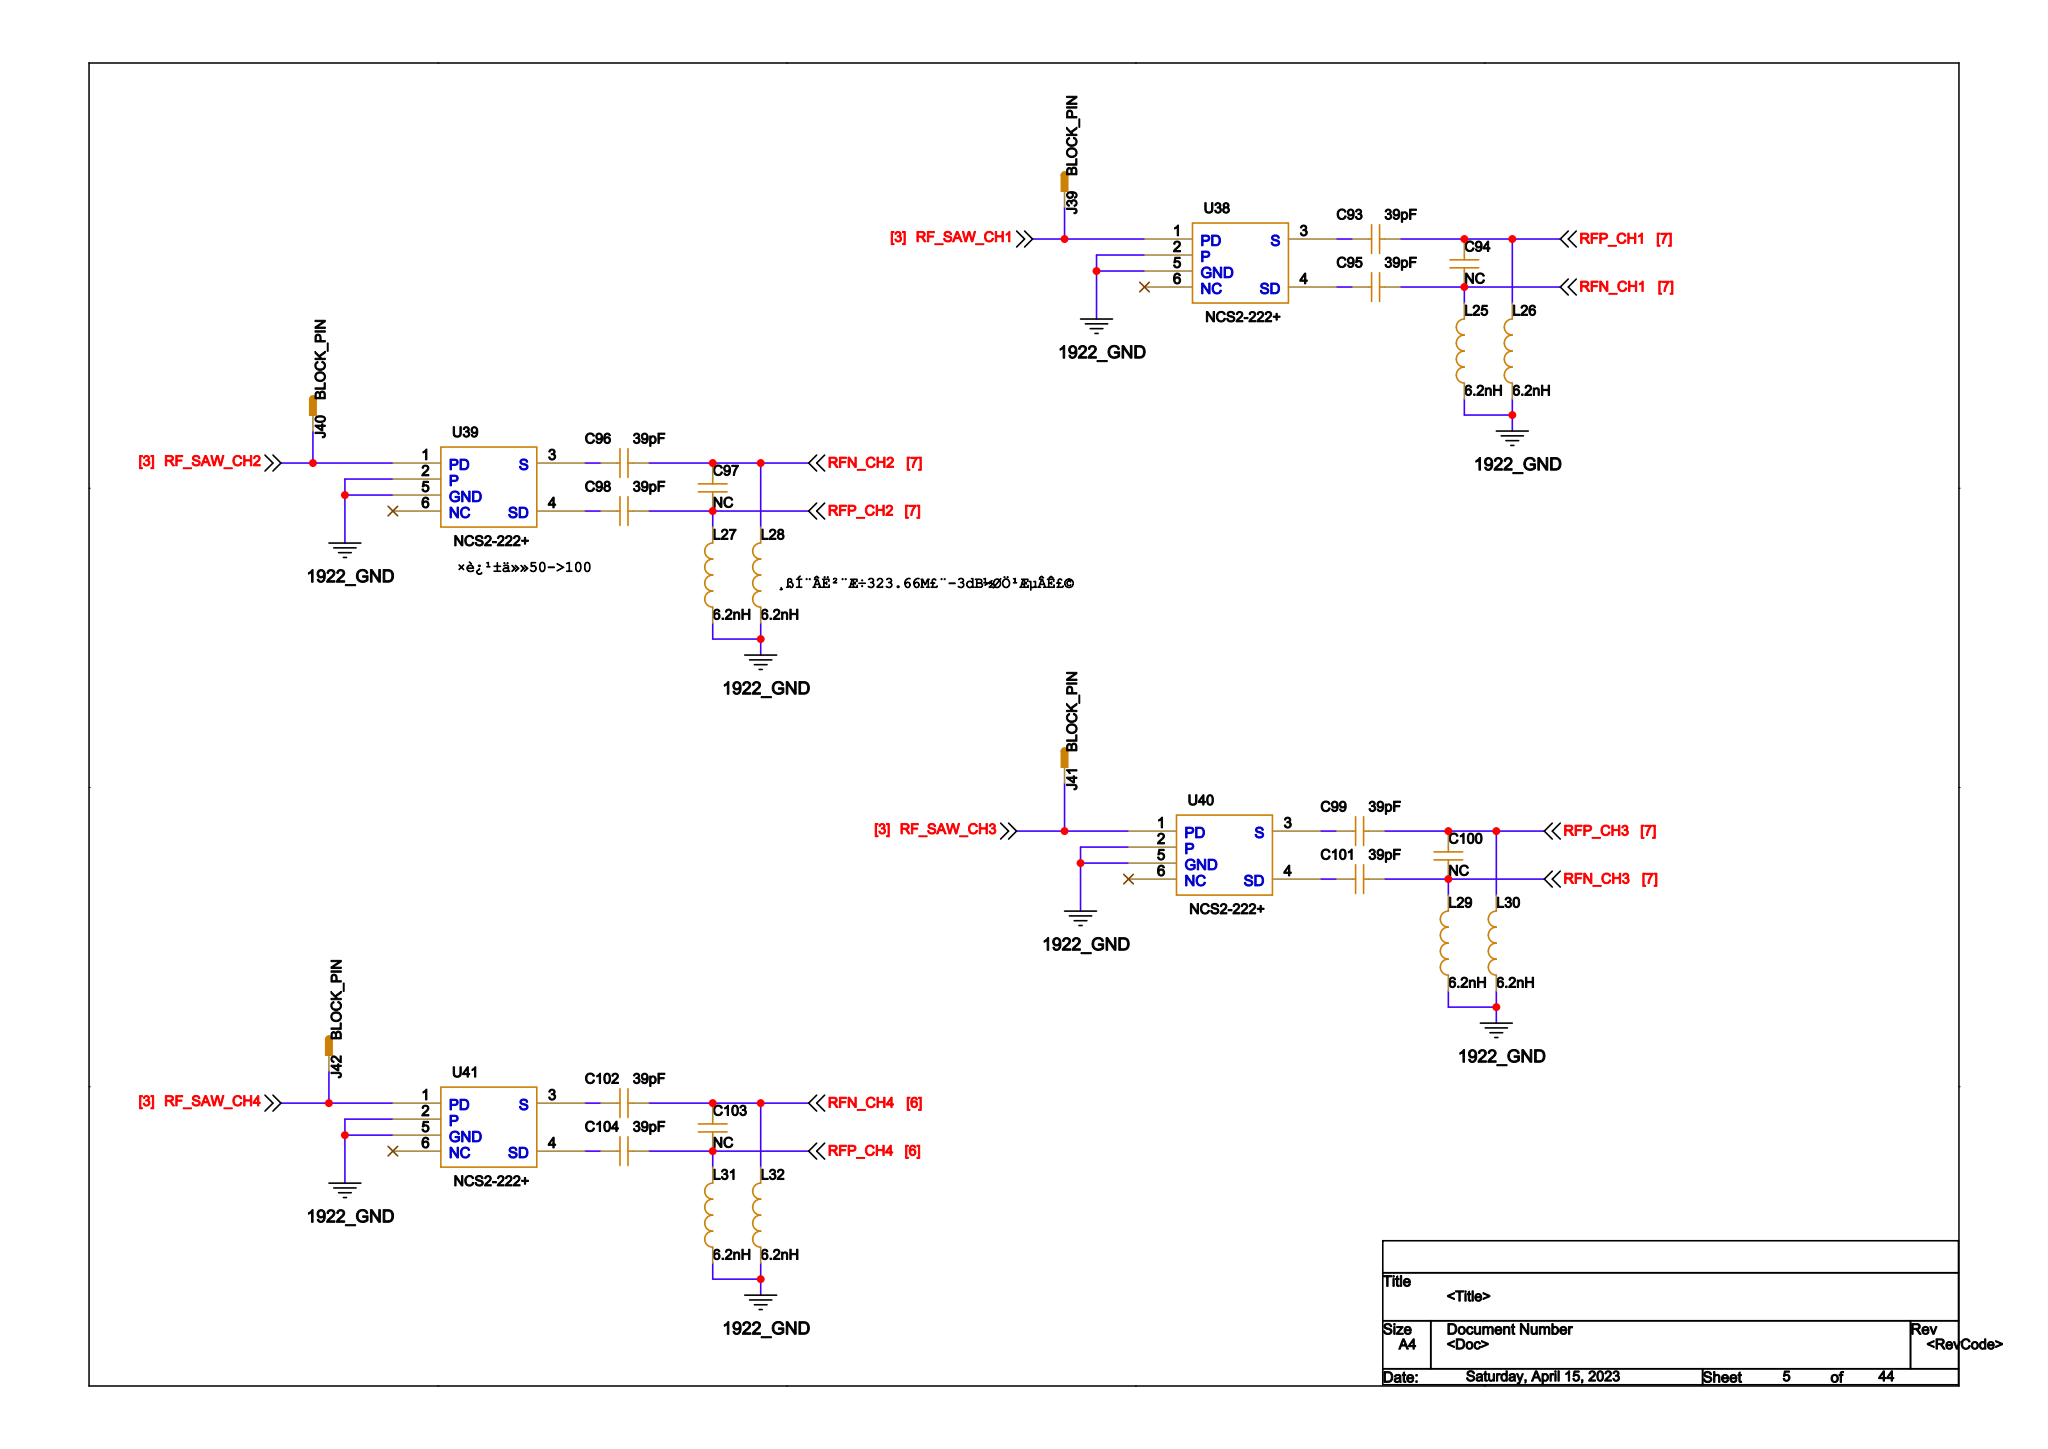Circuit board | Cadence Allegro | 1034 parts | 912 nets | one sheet of the schematic
Parts on this sheet (reference | value | footprint):
C93 | 39pF | C0402
C94 | NC | C0402
C95 | 39pF | C0402
C96 | 39pF | C0402
C97 | NC | C0402
C98 | 39pF | C0402
C99 | 39pF | C0402
C100 | NC | C0402
C101 | 39pF | C0402
C102 | 39pF | C0402
C103 | NC | C0402
C104 | 39pF | C0402
J39 | BLOCK_PIN | B_PIN_SMD
J40 | BLOCK_PIN | B_PIN_SMD
J41 | BLOCK_PIN | B_PIN_SMD
J42 | BLOCK_PIN | B_PIN_SMD
L25 | 6.2nH | L0402
L26 | 6.2nH | L0402
L27 | 6.2nH | L0402
L28 | 6.2nH | L0402
L29 | 6.2nH | L0402
L30 | 6.2nH | L0402
L31 | 6.2nH | L0402
L32 | 6.2nH | L0402
U38 | NCS2-222+ | NCS2_BL_SMD
U39 | NCS2-222+ | NCS2_BL_SMD
U40 | NCS2-222+ | NCS2_BL_SMD
U41 | NCS2-222+ | NCS2_BL_SMD
Nets of these parts (net: part-pin ...):
RF_SAW_CH1_D2: J39-1 U38-1
RF_SAW_CH2_D2: J40-1 U39-1
RF_SAW_CH3_D2: J41-1 U40-1
RF_SAW_CH4_D2: J42-1 U41-1
1922_GND: L25-1 L26-1 L27-1 L28-1 L29-1 L30-1 L31-1 L32-1 U38-2 U38-5 U39-2 U39-5 U40-2 U40-5 U41-2 U41-5
RFN_CH3_D2: C100-1 C101-2 L29-2
RFP_CH3_D2: C99-2 C100-2 L30-2
RFP_CH4_D2: C103-1 C104-2 L31-2
RFN_CH4_D2: C102-2 C103-2 L32-2
RFN_CH1_D2: C94-1 C95-2 L25-2
RFP_CH1_D2: C93-2 C94-2 L26-2
RFP_CH2_D2: C97-1 C98-2 L27-2
RFN_CH2_D2: C96-2 C97-2 L28-2
N437570_D2: C101-1 U40-4
N436601_D2: C102-1 U41-3
N436697_D2: C104-1 U41-4
N435308_D2: C93-1 U38-3
N149989_D2: C95-1 U38-4
N435961_D2: C96-1 U39-3
N436057_D2: C98-1 U39-4
N437474_D2: C99-1 U40-3